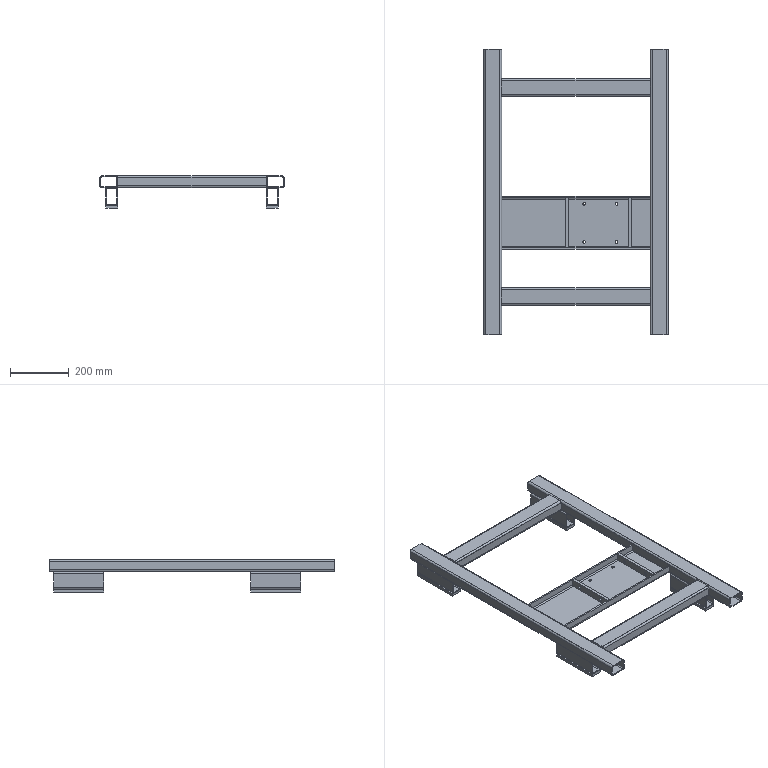Part | STEP file | 15 solids | 254 faces | box 626 x 970 x 110 mm | volume 2991413 mm3 | plane 134 | cylinder 120 | commonest cylinder face diameters 10.2 x40 6.4 x32 12.8 x32 9 x8 8 x6 18 x2